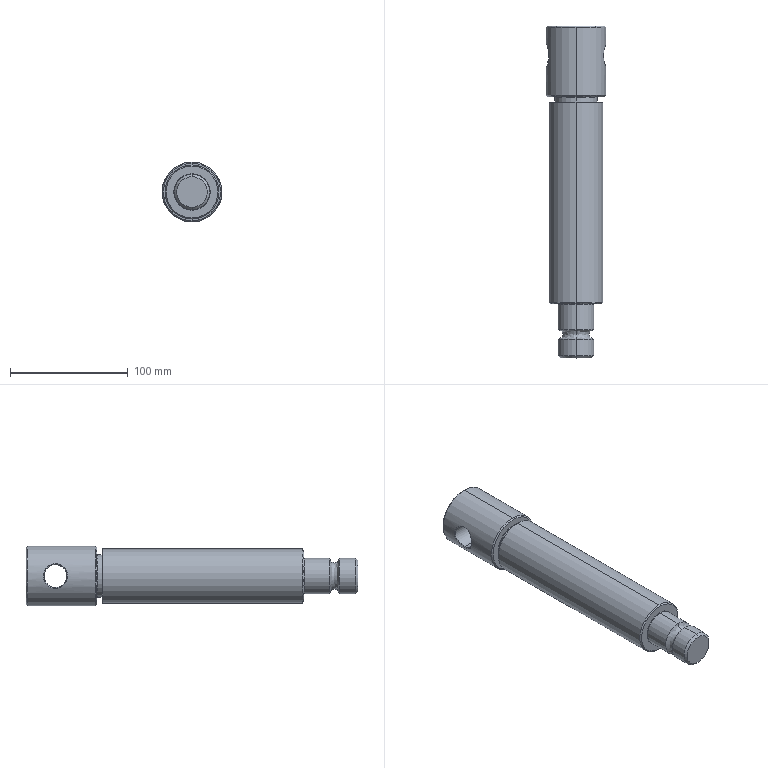Part | SolidWorks | features BaseBody 1 | 1 solid | 37 faces | box 50.8 x 282 x 50.8 mm | volume 426019 mm3 | spline 12 | cylinder 12 | cone 8 | plane 5 | commonest cylinder face diameters 30 x4 19.5 x2 36 x2 46 x2 50.8 x2